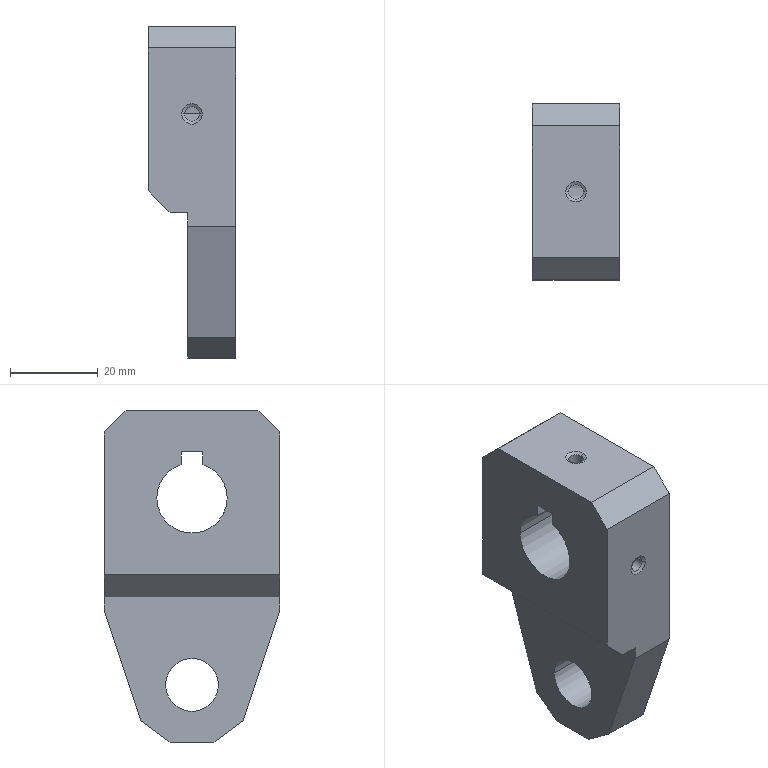Part | NX | 1 solid | 31 faces | box 20 x 40 x 75.5 mm | volume 38243 mm3 | plane 18 | cylinder 9 | cone 4 | commonest cylinder face diameters 3.3 x4 16 x3 12 x2
STEP:
#1=CARTESIAN_POINT('',(1874.,-5.,-55.5));
#2=VERTEX_POINT('',#1);
#3=CARTESIAN_POINT('',(1885.,-5.,-55.5));
#4=VERTEX_POINT('',#3);
#5=CARTESIAN_POINT('',(1879.5,-5.,-55.5));
#6=DIRECTION('',(1.,0.,0.));
#7=VECTOR('',#6,1000.);
#8=LINE('',#5,#7);
#9=EDGE_CURVE('',#2,#4,#8,.T.);
#10=ORIENTED_EDGE('',*,*,#9,.F.);
#11=CARTESIAN_POINT('',(1874.,5.,-55.5));
#12=VERTEX_POINT('',#11);
#13=CARTESIAN_POINT('',(1874.,-0.7647,-55.5));
#14=DIRECTION('',(0.,1.,0.));
#15=VECTOR('',#14,1000.);
#16=LINE('',#13,#15);
#17=EDGE_CURVE('',#2,#12,#16,.T.);
#18=ORIENTED_EDGE('',*,*,#17,.T.);
#19=CARTESIAN_POINT('',(1885.,5.,-55.5));
#20=VERTEX_POINT('',#19);
#21=CARTESIAN_POINT('',(1879.5,5.,-55.5));
#22=DIRECTION('',(-1.,0.,0.));
#23=VECTOR('',#22,1000.);
#24=LINE('',#21,#23);
#25=EDGE_CURVE('',#20,#12,#24,.T.);
#26=ORIENTED_EDGE('',*,*,#25,.F.);
#27=CARTESIAN_POINT('',(1885.,-0.7647,-55.5));
#28=DIRECTION('',(0.,1.,0.));
#29=VECTOR('',#28,1000.);
#30=LINE('',#27,#29);
#31=EDGE_CURVE('',#4,#20,#30,.T.);
#32=ORIENTED_EDGE('',*,*,#31,.F.);
#33=EDGE_LOOP('',(#10,#18,#26,#32));
#34=FACE_BOUND('',#33,.T.);
#35=CARTESIAN_POINT('',(1885.,-20.,-55.5));
#36=DIRECTION('',(0.,0.,-1.));
#37=DIRECTION('',(0.,-1.,0.));
#38=AXIS2_PLACEMENT_3D('',#35,#36,#37);
#39=PLANE('',#38);
#40=ADVANCED_FACE('',(#34),#39,.T.);
#41=CARTESIAN_POINT('',(1865.,-20.,15.));
#42=VERTEX_POINT('',#41);
#43=CARTESIAN_POINT('',(1885.,-20.,15.));
#44=VERTEX_POINT('',#43);
#45=CARTESIAN_POINT('',(0.,-20.,15.));
#46=DIRECTION('',(1.,0.,0.));
#47=VECTOR('',#46,1000.);
#48=LINE('',#45,#47);
#49=EDGE_CURVE('',#42,#44,#48,.T.);
#50=ORIENTED_EDGE('',*,*,#49,.F.);
#51=CARTESIAN_POINT('',(1865.,-20.,-17.5));
#52=VERTEX_POINT('',#51);
#53=CARTESIAN_POINT('',(1865.,-20.,0.));
#54=DIRECTION('',(0.,0.,-1.));
#55=VECTOR('',#54,1000.);
#56=LINE('',#53,#55);
#57=EDGE_CURVE('',#42,#52,#56,.T.);
#58=ORIENTED_EDGE('',*,*,#57,.T.);
#59=CARTESIAN_POINT('',(1870.,-20.,-22.5));
#60=VERTEX_POINT('',#59);
#61=CARTESIAN_POINT('',(1847.5,-20.,0.));
#62=DIRECTION('',(0.7071,0.,-0.7071));
#63=VECTOR('',#62,1000.);
#64=LINE('',#61,#63);
#65=EDGE_CURVE('',#52,#60,#64,.T.);
#66=ORIENTED_EDGE('',*,*,#65,.T.);
#67=CARTESIAN_POINT('',(1874.,-20.,-22.5));
#68=VERTEX_POINT('',#67);
#69=CARTESIAN_POINT('',(0.,-20.,-22.5));
#70=DIRECTION('',(1.,0.,0.));
#71=VECTOR('',#70,1000.);
#72=LINE('',#69,#71);
#73=EDGE_CURVE('',#60,#68,#72,.T.);
#74=ORIENTED_EDGE('',*,*,#73,.T.);
#75=CARTESIAN_POINT('',(1874.,-20.,-25.5));
#76=VERTEX_POINT('',#75);
#77=CARTESIAN_POINT('',(1874.,-20.,0.));
#78=DIRECTION('',(0.,0.,-1.));
#79=VECTOR('',#78,1000.);
#80=LINE('',#77,#79);
#81=EDGE_CURVE('',#68,#76,#80,.T.);
#82=ORIENTED_EDGE('',*,*,#81,.T.);
#83=CARTESIAN_POINT('',(1885.,-20.,-25.5));
#84=VERTEX_POINT('',#83);
#85=CARTESIAN_POINT('',(0.,-20.,-25.5));
#86=DIRECTION('',(1.,0.,0.));
#87=VECTOR('',#86,1000.);
#88=LINE('',#85,#87);
#89=EDGE_CURVE('',#76,#84,#88,.T.);
#90=ORIENTED_EDGE('',*,*,#89,.T.);
#91=CARTESIAN_POINT('',(1885.,-20.,0.));
#92=DIRECTION('',(0.,0.,-1.));
#93=VECTOR('',#92,1000.);
#94=LINE('',#91,#93);
#95=EDGE_CURVE('',#44,#84,#94,.T.);
#96=ORIENTED_EDGE('',*,*,#95,.F.);
#97=EDGE_LOOP('',(#50,#58,#66,#74,#82,#90,#96));
#98=FACE_BOUND('',#97,.T.);
#99=CARTESIAN_POINT('',(1877.315,-20.,0.));
#100=VERTEX_POINT('',#99);
#101=CARTESIAN_POINT('',(1872.685,-20.,0.));
#102=VERTEX_POINT('',#101);
#103=CARTESIAN_POINT('',(1875.,-20.,0.));
#104=DIRECTION('',(0.,-1.,0.));
#105=DIRECTION('',(-1.,0.,0.));
#106=AXIS2_PLACEMENT_3D('',#103,#104,#105);
#107=CIRCLE('',#106,2.315);
#108=EDGE_CURVE('',#100,#102,#107,.T.);
#109=ORIENTED_EDGE('',*,*,#108,.F.);
#110=CARTESIAN_POINT('',(1875.,-20.,0.));
#111=DIRECTION('',(0.,-1.,0.));
#112=DIRECTION('',(-1.,0.,0.));
#113=AXIS2_PLACEMENT_3D('',#110,#111,#112);
#114=CIRCLE('',#113,2.315);
#115=EDGE_CURVE('',#102,#100,#114,.T.);
#116=ORIENTED_EDGE('',*,*,#115,.F.);
#117=EDGE_LOOP('',(#109,#116));
#118=FACE_BOUND('',#117,.T.);
#119=CARTESIAN_POINT('',(1885.,-20.,20.));
#120=DIRECTION('',(0.,-1.,0.));
#121=DIRECTION('',(0.,0.,-1.));
#122=AXIS2_PLACEMENT_3D('',#119,#120,#121);
#123=PLANE('',#122);
#124=ADVANCED_FACE('',(#98,#118),#123,.T.);
#125=CARTESIAN_POINT('',(1865.,15.,20.));
#126=VERTEX_POINT('',#125);
#127=CARTESIAN_POINT('',(1885.,15.,20.));
#128=VERTEX_POINT('',#127);
#129=CARTESIAN_POINT('',(0.,15.,20.));
#130=DIRECTION('',(1.,0.,0.));
#131=VECTOR('',#130,1000.);
#132=LINE('',#129,#131);
#133=EDGE_CURVE('',#126,#128,#132,.T.);
#134=ORIENTED_EDGE('',*,*,#133,.F.);
#135=CARTESIAN_POINT('',(1865.,-15.,20.));
#136=VERTEX_POINT('',#135);
#137=CARTESIAN_POINT('',(1865.,0.,20.));
#138=DIRECTION('',(0.,-1.,0.));
#139=VECTOR('',#138,1000.);
#140=LINE('',#137,#139);
#141=EDGE_CURVE('',#126,#136,#140,.T.);
#142=ORIENTED_EDGE('',*,*,#141,.T.);
#143=CARTESIAN_POINT('',(1885.,-15.,20.));
#144=VERTEX_POINT('',#143);
#145=CARTESIAN_POINT('',(0.,-15.,20.));
#146=DIRECTION('',(-1.,0.,0.));
#147=VECTOR('',#146,1000.);
#148=LINE('',#145,#147);
#149=EDGE_CURVE('',#144,#136,#148,.T.);
#150=ORIENTED_EDGE('',*,*,#149,.F.);
#151=CARTESIAN_POINT('',(1885.,0.,20.));
#152=DIRECTION('',(0.,-1.,0.));
#153=VECTOR('',#152,1000.);
#154=LINE('',#151,#153);
#155=EDGE_CURVE('',#128,#144,#154,.T.);
#156=ORIENTED_EDGE('',*,*,#155,.F.);
#157=EDGE_LOOP('',(#134,#142,#150,#156));
#158=FACE_BOUND('',#157,.T.);
#159=CARTESIAN_POINT('',(1872.685,0.,20.));
#160=VERTEX_POINT('',#159);
#161=CARTESIAN_POINT('',(1877.315,0.,20.));
#162=VERTEX_POINT('',#161);
#163=CARTESIAN_POINT('',(1875.,0.,20.));
#164=DIRECTION('',(0.,0.,1.));
#165=DIRECTION('',(1.,0.,0.));
#166=AXIS2_PLACEMENT_3D('',#163,#164,#165);
#167=CIRCLE('',#166,2.315);
#168=EDGE_CURVE('',#160,#162,#167,.T.);
#169=ORIENTED_EDGE('',*,*,#168,.F.);
#170=CARTESIAN_POINT('',(1875.,0.,20.));
#171=DIRECTION('',(0.,0.,1.));
#172=DIRECTION('',(1.,0.,0.));
#173=AXIS2_PLACEMENT_3D('',#170,#171,#172);
#174=CIRCLE('',#173,2.315);
#175=EDGE_CURVE('',#162,#160,#174,.T.);
#176=ORIENTED_EDGE('',*,*,#175,.F.);
#177=EDGE_LOOP('',(#169,#176));
#178=FACE_BOUND('',#177,.T.);
#179=CARTESIAN_POINT('',(1885.,20.,20.));
#180=DIRECTION('',(0.,0.,1.));
#181=DIRECTION('',(1.,0.,0.));
#182=AXIS2_PLACEMENT_3D('',#179,#180,#181);
#183=PLANE('',#182);
#184=ADVANCED_FACE('',(#158,#178),#183,.T.);
#185=CARTESIAN_POINT('',(1870.,20.,-22.5));
#186=VERTEX_POINT('',#185);
#187=CARTESIAN_POINT('',(1874.,20.,-22.5));
#188=VERTEX_POINT('',#187);
#189=CARTESIAN_POINT('',(1885.,20.,-22.5));
#190=DIRECTION('',(1.,0.,0.));
#191=VECTOR('',#190,1000.);
#192=LINE('',#189,#191);
#193=EDGE_CURVE('',#186,#188,#192,.T.);
#194=ORIENTED_EDGE('',*,*,#193,.F.);
#195=CARTESIAN_POINT('',(1865.,20.,-17.5));
#196=VERTEX_POINT('',#195);
#197=CARTESIAN_POINT('',(1885.,20.,-37.5));
#198=DIRECTION('',(-0.7071,0.,0.7071));
#199=VECTOR('',#198,1000.);
#200=LINE('',#197,#199);
#201=EDGE_CURVE('',#186,#196,#200,.T.);
#202=ORIENTED_EDGE('',*,*,#201,.T.);
#203=CARTESIAN_POINT('',(1865.,20.,15.));
#204=VERTEX_POINT('',#203);
#205=CARTESIAN_POINT('',(1865.,20.,0.8535));
#206=DIRECTION('',(0.,0.,1.));
#207=VECTOR('',#206,1000.);
#208=LINE('',#205,#207);
#209=EDGE_CURVE('',#196,#204,#208,.T.);
#210=ORIENTED_EDGE('',*,*,#209,.T.);
#211=CARTESIAN_POINT('',(1885.,20.,15.));
#212=VERTEX_POINT('',#211);
#213=CARTESIAN_POINT('',(1875.,20.,15.));
#214=DIRECTION('',(-1.,0.,0.));
#215=VECTOR('',#214,1000.);
#216=LINE('',#213,#215);
#217=EDGE_CURVE('',#212,#204,#216,.T.);
#218=ORIENTED_EDGE('',*,*,#217,.F.);
#219=CARTESIAN_POINT('',(1885.,20.,-25.5));
#220=VERTEX_POINT('',#219);
#221=CARTESIAN_POINT('',(1885.,20.,0.8535));
#222=DIRECTION('',(0.,0.,1.));
#223=VECTOR('',#222,1000.);
#224=LINE('',#221,#223);
#225=EDGE_CURVE('',#220,#212,#224,.T.);
#226=ORIENTED_EDGE('',*,*,#225,.F.);
#227=CARTESIAN_POINT('',(1874.,20.,-25.5));
#228=VERTEX_POINT('',#227);
#229=CARTESIAN_POINT('',(1879.5,20.,-25.5));
#230=DIRECTION('',(-1.,0.,0.));
#231=VECTOR('',#230,1000.);
#232=LINE('',#229,#231);
#233=EDGE_CURVE('',#220,#228,#232,.T.);
#234=ORIENTED_EDGE('',*,*,#233,.T.);
#235=CARTESIAN_POINT('',(1874.,20.,0.8535));
#236=DIRECTION('',(0.,0.,1.));
#237=VECTOR('',#236,1000.);
#238=LINE('',#235,#237);
#239=EDGE_CURVE('',#228,#188,#238,.T.);
#240=ORIENTED_EDGE('',*,*,#239,.T.);
#241=EDGE_LOOP('',(#194,#202,#210,#218,#226,#234,#240));
#242=FACE_BOUND('',#241,.T.);
#243=CARTESIAN_POINT('',(1885.,20.,-62.5));
#244=DIRECTION('',(0.,1.,0.));
#245=DIRECTION('',(1.,0.,0.));
#246=AXIS2_PLACEMENT_3D('',#243,#244,#245);
#247=PLANE('',#246);
#248=ADVANCED_FACE('',(#242),#247,.T.);
#249=CARTESIAN_POINT('',(1870.,0.,-22.5));
#250=DIRECTION('',(0.,-1.,0.));
#251=VECTOR('',#250,1000.);
#252=LINE('',#249,#251);
#253=EDGE_CURVE('',#186,#60,#252,.T.);
#254=ORIENTED_EDGE('',*,*,#253,.F.);
#255=ORIENTED_EDGE('',*,*,#193,.T.);
#256=CARTESIAN_POINT('',(1874.,24.,-22.5));
#257=DIRECTION('',(0.,-1.,0.));
#258=VECTOR('',#257,1000.);
#259=LINE('',#256,#258);
#260=EDGE_CURVE('',#188,#68,#259,.T.);
#261=ORIENTED_EDGE('',*,*,#260,.T.);
#262=ORIENTED_EDGE('',*,*,#73,.F.);
#263=EDGE_LOOP('',(#254,#255,#261,#262));
#264=FACE_BOUND('',#263,.T.);
#265=CARTESIAN_POINT('',(1865.,24.,-22.5));
#266=DIRECTION('',(0.,0.,1.));
#267=DIRECTION('',(1.,0.,0.));
#268=AXIS2_PLACEMENT_3D('',#265,#266,#267);
#269=PLANE('',#268);
#270=ADVANCED_FACE('',(#264),#269,.F.);
#271=ORIENTED_EDGE('',*,*,#133,.T.);
#272=CARTESIAN_POINT('',(1885.,34.147,0.8535));
#273=DIRECTION('',(0.,0.7071,-0.7071));
#274=VECTOR('',#273,1000.);
#275=LINE('',#272,#274);
#276=EDGE_CURVE('',#128,#212,#275,.T.);
#277=ORIENTED_EDGE('',*,*,#276,.T.);
#278=ORIENTED_EDGE('',*,*,#217,.T.);
#279=CARTESIAN_POINT('',(1865.,34.147,0.8535));
#280=DIRECTION('',(0.,0.7071,-0.7071));
#281=VECTOR('',#280,1000.);
#282=LINE('',#279,#281);
#283=EDGE_CURVE('',#126,#204,#282,.T.);
#284=ORIENTED_EDGE('',*,*,#283,.F.);
#285=EDGE_LOOP('',(#271,#277,#278,#284));
#286=FACE_BOUND('',#285,.T.);
#287=CARTESIAN_POINT('',(1875.,17.5,17.5));
#288=DIRECTION('',(0.,0.7071,0.7071));
#289=DIRECTION('',(1.,0.,0.));
#290=AXIS2_PLACEMENT_3D('',#287,#288,#289);
#291=PLANE('',#290);
#292=ADVANCED_FACE('',(#286),#291,.T.);
#293=ORIENTED_EDGE('',*,*,#253,.T.);
#294=ORIENTED_EDGE('',*,*,#65,.F.);
#295=CARTESIAN_POINT('',(1865.,0.,-17.5));
#296=DIRECTION('',(0.,-1.,0.));
#297=VECTOR('',#296,1000.);
#298=LINE('',#295,#297);
#299=EDGE_CURVE('',#196,#52,#298,.T.);
#300=ORIENTED_EDGE('',*,*,#299,.F.);
#301=ORIENTED_EDGE('',*,*,#201,.F.);
#302=EDGE_LOOP('',(#293,#294,#300,#301));
#303=FACE_BOUND('',#302,.T.);
#304=CARTESIAN_POINT('',(1867.5,0.,-20.));
#305=DIRECTION('',(0.7071,0.,0.7071));
#306=DIRECTION('',(0.,-1.,0.));
#307=AXIS2_PLACEMENT_3D('',#304,#305,#306);
#308=PLANE('',#307);
#309=ADVANCED_FACE('',(#303),#308,.F.);
#310=CARTESIAN_POINT('',(1865.,2.5,7.599));
#311=VERTEX_POINT('',#310);
#312=CARTESIAN_POINT('',(1885.,2.5,7.599));
#313=VERTEX_POINT('',#312);
#314=CARTESIAN_POINT('',(1885.,2.5,7.599));
#315=DIRECTION('',(1.,0.,0.));
#316=VECTOR('',#315,1000.);
#317=LINE('',#314,#316);
#318=EDGE_CURVE('',#311,#313,#317,.T.);
#319=ORIENTED_EDGE('',*,*,#318,.T.);
#320=CARTESIAN_POINT('',(1885.,2.5,10.5));
#321=VERTEX_POINT('',#320);
#322=CARTESIAN_POINT('',(1885.,2.5,0.8535));
#323=DIRECTION('',(0.,0.,1.));
#324=VECTOR('',#323,1000.);
#325=LINE('',#322,#324);
#326=EDGE_CURVE('',#313,#321,#325,.T.);
#327=ORIENTED_EDGE('',*,*,#326,.T.);
#328=CARTESIAN_POINT('',(1865.,2.5,10.5));
#329=VERTEX_POINT('',#328);
#330=CARTESIAN_POINT('',(0.,2.5,10.5));
#331=DIRECTION('',(1.,0.,0.));
#332=VECTOR('',#331,1000.);
#333=LINE('',#330,#332);
#334=EDGE_CURVE('',#329,#321,#333,.T.);
#335=ORIENTED_EDGE('',*,*,#334,.F.);
#336=CARTESIAN_POINT('',(1865.,2.5,0.8535));
#337=DIRECTION('',(0.,0.,1.));
#338=VECTOR('',#337,1000.);
#339=LINE('',#336,#338);
#340=EDGE_CURVE('',#311,#329,#339,.T.);
#341=ORIENTED_EDGE('',*,*,#340,.F.);
#342=EDGE_LOOP('',(#319,#327,#335,#341));
#343=FACE_BOUND('',#342,.T.);
#344=CARTESIAN_POINT('',(1863.,2.5,10.5));
#345=DIRECTION('',(0.,1.,0.));
#346=DIRECTION('',(1.,0.,0.));
#347=AXIS2_PLACEMENT_3D('',#344,#345,#346);
#348=PLANE('',#347);
#349=ADVANCED_FACE('',(#343),#348,.F.);
#350=CARTESIAN_POINT('',(1885.,6.,-42.5));
#351=VERTEX_POINT('',#350);
#352=CARTESIAN_POINT('',(1885.,-6.,-42.5));
#353=VERTEX_POINT('',#352);
#354=CARTESIAN_POINT('',(1885.,0.,-42.5));
#355=DIRECTION('',(1.,0.,0.));
#356=DIRECTION('',(0.,1.,0.));
#357=AXIS2_PLACEMENT_3D('',#354,#355,#356);
#358=CIRCLE('',#357,6.);
#359=EDGE_CURVE('',#351,#353,#358,.T.);
#360=ORIENTED_EDGE('',*,*,#359,.T.);
#361=CARTESIAN_POINT('',(1874.,-6.,-42.5));
#362=VERTEX_POINT('',#361);
#363=CARTESIAN_POINT('',(1863.,-6.,-42.5));
#364=DIRECTION('',(1.,0.,0.));
#365=VECTOR('',#364,1000.);
#366=LINE('',#363,#365);
#367=EDGE_CURVE('',#353,#362,#366,.F.);
#368=ORIENTED_EDGE('',*,*,#367,.T.);
#369=CARTESIAN_POINT('',(1874.,6.,-42.5));
#370=VERTEX_POINT('',#369);
#371=CARTESIAN_POINT('',(1874.,0.,-42.5));
#372=DIRECTION('',(1.,0.,0.));
#373=DIRECTION('',(0.,1.,0.));
#374=AXIS2_PLACEMENT_3D('',#371,#372,#373);
#375=CIRCLE('',#374,6.);
#376=EDGE_CURVE('',#370,#362,#375,.T.);
#377=ORIENTED_EDGE('',*,*,#376,.F.);
#378=CARTESIAN_POINT('',(1863.,6.,-42.5));
#379=DIRECTION('',(1.,0.,0.));
#380=VECTOR('',#379,1000.);
#381=LINE('',#378,#380);
#382=EDGE_CURVE('',#351,#370,#381,.F.);
#383=ORIENTED_EDGE('',*,*,#382,.F.);
#384=EDGE_LOOP('',(#360,#368,#377,#383));
#385=FACE_BOUND('',#384,.T.);
#386=CARTESIAN_POINT('',(1863.,0.,-42.5));
#387=DIRECTION('',(1.,0.,0.));
#388=DIRECTION('',(0.,1.,0.));
#389=AXIS2_PLACEMENT_3D('',#386,#387,#388);
#390=CYLINDRICAL_SURFACE('',#389,6.);
#391=ADVANCED_FACE('',(#385),#390,.F.);
#392=CARTESIAN_POINT('',(1865.,-8.,0.));
#393=VERTEX_POINT('',#392);
#394=CARTESIAN_POINT('',(1873.35,-8.,0.));
#395=VERTEX_POINT('',#394);
#396=CARTESIAN_POINT('',(1885.,-8.,0.));
#397=DIRECTION('',(1.,0.,0.));
#398=VECTOR('',#397,1000.);
#399=LINE('',#396,#398);
#400=EDGE_CURVE('',#393,#395,#399,.T.);
#401=ORIENTED_EDGE('',*,*,#400,.F.);
#402=CARTESIAN_POINT('',(1865.,-2.5,7.599));
#403=VERTEX_POINT('',#402);
#404=CARTESIAN_POINT('',(1865.,0.,0.));
#405=DIRECTION('',(1.,0.,0.));
#406=DIRECTION('',(0.,1.,0.));
#407=AXIS2_PLACEMENT_3D('',#404,#405,#406);
#408=CIRCLE('',#407,8.);
#409=EDGE_CURVE('',#403,#393,#408,.T.);
#410=ORIENTED_EDGE('',*,*,#409,.F.);
#411=CARTESIAN_POINT('',(1885.,-2.5,7.599));
#412=VERTEX_POINT('',#411);
#413=CARTESIAN_POINT('',(1885.,-2.5,7.599));
#414=DIRECTION('',(1.,0.,0.));
#415=VECTOR('',#414,1000.);
#416=LINE('',#413,#415);
#417=EDGE_CURVE('',#403,#412,#416,.T.);
#418=ORIENTED_EDGE('',*,*,#417,.T.);
#419=CARTESIAN_POINT('',(1885.,-8.,0.));
#420=VERTEX_POINT('',#419);
#421=CARTESIAN_POINT('',(1885.,0.,0.));
#422=DIRECTION('',(1.,0.,0.));
#423=DIRECTION('',(0.,1.,0.));
#424=AXIS2_PLACEMENT_3D('',#421,#422,#423);
#425=CIRCLE('',#424,8.);
#426=EDGE_CURVE('',#412,#420,#425,.T.);
#427=ORIENTED_EDGE('',*,*,#426,.T.);
#428=CARTESIAN_POINT('',(1876.65,-8.,0.));
#429=VERTEX_POINT('',#428);
#430=CARTESIAN_POINT('',(1885.,-8.,0.));
#431=DIRECTION('',(1.,0.,0.));
#432=VECTOR('',#431,1000.);
#433=LINE('',#430,#432);
#434=EDGE_CURVE('',#429,#420,#433,.T.);
#435=ORIENTED_EDGE('',*,*,#434,.F.);
#436=CARTESIAN_POINT('',(1875.,-7.828,1.65));
#437=VERTEX_POINT('',#436);
#438=CARTESIAN_POINT('',(1876.65,-8.,0.));
#439=CARTESIAN_POINT('',(1876.65,-8.,0.05388));
#440=CARTESIAN_POINT('',(1876.647,-7.999,0.1078));
#441=CARTESIAN_POINT('',(1876.642,-7.998,0.1614));
#442=CARTESIAN_POINT('',(1876.639,-7.998,0.1882));
#443=CARTESIAN_POINT('',(1876.636,-7.997,0.2149));
#444=CARTESIAN_POINT('',(1876.632,-7.996,0.2416));
#445=CARTESIAN_POINT('',(1876.628,-7.996,0.2682));
#446=CARTESIAN_POINT('',(1876.624,-7.995,0.2948));
#447=CARTESIAN_POINT('',(1876.618,-7.994,0.3212));
#448=CARTESIAN_POINT('',(1876.613,-7.992,0.3476));
#449=CARTESIAN_POINT('',(1876.607,-7.991,0.3739));
#450=CARTESIAN_POINT('',(1876.601,-7.99,0.4));
#451=CARTESIAN_POINT('',(1876.594,-7.989,0.4262));
#452=CARTESIAN_POINT('',(1876.587,-7.987,0.4522));
#453=CARTESIAN_POINT('',(1876.579,-7.986,0.4779));
#454=CARTESIAN_POINT('',(1876.571,-7.984,0.5037));
#455=CARTESIAN_POINT('',(1876.563,-7.983,0.5292));
#456=CARTESIAN_POINT('',(1876.554,-7.981,0.5546));
#457=CARTESIAN_POINT('',(1876.545,-7.979,0.5799));
#458=CARTESIAN_POINT('',(1876.535,-7.977,0.6051));
#459=CARTESIAN_POINT('',(1876.525,-7.975,0.63));
#460=CARTESIAN_POINT('',(1876.515,-7.973,0.655));
#461=CARTESIAN_POINT('',(1876.504,-7.971,0.6797));
#462=CARTESIAN_POINT('',(1876.492,-7.969,0.7042));
#463=CARTESIAN_POINT('',(1876.481,-7.967,0.7287));
#464=CARTESIAN_POINT('',(1876.468,-7.965,0.7529));
#465=CARTESIAN_POINT('',(1876.456,-7.962,0.7768));
#466=CARTESIAN_POINT('',(1876.443,-7.96,0.8007));
#467=CARTESIAN_POINT('',(1876.43,-7.957,0.8242));
#468=CARTESIAN_POINT('',(1876.416,-7.955,0.8475));
#469=CARTESIAN_POINT('',(1876.402,-7.953,0.8707));
#470=CARTESIAN_POINT('',(1876.387,-7.95,0.8936));
#471=CARTESIAN_POINT('',(1876.372,-7.947,0.9161));
#472=CARTESIAN_POINT('',(1876.357,-7.945,0.9386));
#473=CARTESIAN_POINT('',(1876.342,-7.942,0.9607));
#474=CARTESIAN_POINT('',(1876.326,-7.939,0.9824));
#475=CARTESIAN_POINT('',(1876.31,-7.937,1.004));
#476=CARTESIAN_POINT('',(1876.293,-7.934,1.025));
#477=CARTESIAN_POINT('',(1876.276,-7.931,1.046));
#478=CARTESIAN_POINT('',(1876.259,-7.929,1.067));
#479=CARTESIAN_POINT('',(1876.242,-7.926,1.087));
#480=CARTESIAN_POINT('',(1876.224,-7.923,1.107));
#481=CARTESIAN_POINT('',(1876.206,-7.92,1.127));
#482=CARTESIAN_POINT('',(1876.187,-7.917,1.146));
#483=CARTESIAN_POINT('',(1876.168,-7.915,1.166));
#484=CARTESIAN_POINT('',(1876.149,-7.912,1.185));
#485=CARTESIAN_POINT('',(1876.129,-7.909,1.203));
#486=CARTESIAN_POINT('',(1876.109,-7.906,1.221));
#487=CARTESIAN_POINT('',(1876.089,-7.903,1.24));
#488=CARTESIAN_POINT('',(1876.069,-7.901,1.257));
#489=CARTESIAN_POINT('',(1876.048,-7.898,1.274));
#490=CARTESIAN_POINT('',(1876.027,-7.895,1.292));
#491=CARTESIAN_POINT('',(1876.006,-7.892,1.308));
#492=CARTESIAN_POINT('',(1875.984,-7.89,1.324));
#493=CARTESIAN_POINT('',(1875.962,-7.887,1.341));
#494=CARTESIAN_POINT('',(1875.94,-7.884,1.356));
#495=CARTESIAN_POINT('',(1875.918,-7.882,1.371));
#496=CARTESIAN_POINT('',(1875.895,-7.879,1.386));
#497=CARTESIAN_POINT('',(1875.872,-7.876,1.401));
#498=CARTESIAN_POINT('',(1875.849,-7.874,1.415));
#499=CARTESIAN_POINT('',(1875.826,-7.871,1.429));
#500=CARTESIAN_POINT('',(1875.803,-7.869,1.442));
#501=CARTESIAN_POINT('',(1875.779,-7.867,1.455));
#502=CARTESIAN_POINT('',(1875.755,-7.864,1.467));
#503=CARTESIAN_POINT('',(1875.731,-7.862,1.479));
#504=CARTESIAN_POINT('',(1875.707,-7.86,1.491));
#505=CARTESIAN_POINT('',(1875.683,-7.858,1.502));
#506=CARTESIAN_POINT('',(1875.658,-7.856,1.513));
#507=CARTESIAN_POINT('',(1875.633,-7.854,1.524));
#508=CARTESIAN_POINT('',(1875.608,-7.852,1.534));
#509=CARTESIAN_POINT('',(1875.583,-7.85,1.544));
#510=CARTESIAN_POINT('',(1875.557,-7.848,1.553));
#511=CARTESIAN_POINT('',(1875.532,-7.846,1.562));
#512=CARTESIAN_POINT('',(1875.506,-7.844,1.571));
#513=CARTESIAN_POINT('',(1875.48,-7.843,1.579));
#514=CARTESIAN_POINT('',(1875.454,-7.841,1.586));
#515=CARTESIAN_POINT('',(1875.428,-7.84,1.594));
#516=CARTESIAN_POINT('',(1875.402,-7.838,1.6));
#517=CARTESIAN_POINT('',(1875.375,-7.837,1.607));
#518=CARTESIAN_POINT('',(1875.349,-7.836,1.613));
#519=CARTESIAN_POINT('',(1875.322,-7.835,1.618));
#520=CARTESIAN_POINT('',(1875.296,-7.834,1.624));
#521=CARTESIAN_POINT('',(1875.269,-7.833,1.628));
#522=CARTESIAN_POINT('',(1875.242,-7.832,1.632));
#523=CARTESIAN_POINT('',(1875.215,-7.831,1.636));
#524=CARTESIAN_POINT('',(1875.188,-7.83,1.639));
#525=CARTESIAN_POINT('',(1875.161,-7.83,1.642));
#526=CARTESIAN_POINT('',(1875.135,-7.829,1.645));
#527=CARTESIAN_POINT('',(1875.108,-7.829,1.647));
#528=CARTESIAN_POINT('',(1875.081,-7.828,1.648));
#529=CARTESIAN_POINT('',(1875.054,-7.828,1.649));
#530=CARTESIAN_POINT('',(1875.027,-7.828,1.65));
#531=CARTESIAN_POINT('',(1875.,-7.828,1.65));
#532=B_SPLINE_CURVE_WITH_KNOTS('',3,(#438,#439,#440,#441,#442,#443,#444,#445,#446,#447,#448,#449,#450,#451,#452,#453,#454,#455,#456,#457,#458,#459,#460,#461,#462,#463,#464,#465,#466,#467,#468,#469,#470,#471,#472,#473,#474,#475,#476,#477,#478,#479,#480,#481,#482,#483,#484,#485,#486,#487,#488,#489,#490,#491,#492,#493,#494,#495,#496,#497,#498,#499,#500,#501,#502,#503,#504,#505,#506,#507,#508,#509,#510,#511,#512,#513,#514,#515,#516,#517,#518,#519,#520,#521,#522,#523,#524,#525,#526,#527,#528,#529,#530,#531),.UNSPECIFIED.,.F.,.F.,(4,3,3,3,3,3,3,3,3,3,3,3,3,3,3,3,3,3,3,3,3,3,3,3,3,3,3,3,3,3,3,4),(0.,0.1617,0.2425,0.3233,0.4042,0.4852,0.566,0.6471,0.7284,0.8099,0.8915,0.973,1.054,1.136,1.217,1.298,1.379,1.461,1.542,1.624,1.705,1.786,1.867,1.948,2.03,2.111,2.193,2.274,2.356,2.437,2.518,2.599),.UNSPECIFIED.);
#533=EDGE_CURVE('',#429,#437,#532,.T.);
#534=ORIENTED_EDGE('',*,*,#533,.T.);
#535=CARTESIAN_POINT('',(1875.,-7.828,1.65));
#536=CARTESIAN_POINT('',(1874.973,-7.828,1.65));
#537=CARTESIAN_POINT('',(1874.946,-7.828,1.649));
#538=CARTESIAN_POINT('',(1874.919,-7.828,1.648));
#539=CARTESIAN_POINT('',(1874.892,-7.829,1.647));
#540=CARTESIAN_POINT('',(1874.865,-7.829,1.645));
#541=CARTESIAN_POINT('',(1874.838,-7.83,1.642));
#542=CARTESIAN_POINT('',(1874.811,-7.83,1.639));
#543=CARTESIAN_POINT('',(1874.784,-7.831,1.636));
#544=CARTESIAN_POINT('',(1874.757,-7.832,1.632));
#545=CARTESIAN_POINT('',(1874.73,-7.833,1.628));
#546=CARTESIAN_POINT('',(1874.704,-7.834,1.623));
#547=CARTESIAN_POINT('',(1874.677,-7.835,1.618));
#548=CARTESIAN_POINT('',(1874.65,-7.836,1.613));
#549=CARTESIAN_POINT('',(1874.624,-7.837,1.607));
#550=CARTESIAN_POINT('',(1874.597,-7.838,1.6));
#551=CARTESIAN_POINT('',(1874.571,-7.84,1.594));
#552=CARTESIAN_POINT('',(1874.545,-7.841,1.586));
#553=CARTESIAN_POINT('',(1874.519,-7.843,1.578));
#554=CARTESIAN_POINT('',(1874.493,-7.844,1.57));
#555=CARTESIAN_POINT('',(1874.467,-7.846,1.562));
#556=CARTESIAN_POINT('',(1874.442,-7.848,1.553));
#557=CARTESIAN_POINT('',(1874.417,-7.85,1.544));
#558=CARTESIAN_POINT('',(1874.392,-7.852,1.534));
#559=CARTESIAN_POINT('',(1874.367,-7.854,1.524));
#560=CARTESIAN_POINT('',(1874.342,-7.856,1.513));
#561=CARTESIAN_POINT('',(1874.317,-7.858,1.502));
#562=CARTESIAN_POINT('',(1874.293,-7.86,1.491));
#563=CARTESIAN_POINT('',(1874.269,-7.862,1.479));
#564=CARTESIAN_POINT('',(1874.245,-7.864,1.467));
#565=CARTESIAN_POINT('',(1874.221,-7.867,1.454));
#566=CARTESIAN_POINT('',(1874.197,-7.869,1.442));
#567=CARTESIAN_POINT('',(1874.173,-7.871,1.428));
#568=CARTESIAN_POINT('',(1874.15,-7.874,1.414));
#569=CARTESIAN_POINT('',(1874.127,-7.877,1.4));
#570=CARTESIAN_POINT('',(1874.104,-7.879,1.386));
#571=CARTESIAN_POINT('',(1874.082,-7.882,1.371));
#572=CARTESIAN_POINT('',(1874.059,-7.884,1.356));
#573=CARTESIAN_POINT('',(1874.037,-7.887,1.34));
#574=CARTESIAN_POINT('',(1874.015,-7.89,1.324));
#575=CARTESIAN_POINT('',(1873.994,-7.892,1.308));
#576=CARTESIAN_POINT('',(1873.972,-7.895,1.291));
#577=CARTESIAN_POINT('',(1873.951,-7.898,1.274));
#578=CARTESIAN_POINT('',(1873.931,-7.901,1.257));
#579=CARTESIAN_POINT('',(1873.91,-7.903,1.239));
#580=CARTESIAN_POINT('',(1873.89,-7.906,1.221));
#581=CARTESIAN_POINT('',(1873.87,-7.909,1.203));
#582=CARTESIAN_POINT('',(1873.851,-7.912,1.184));
#583=CARTESIAN_POINT('',(1873.832,-7.915,1.165));
#584=CARTESIAN_POINT('',(1873.813,-7.917,1.146));
#585=CARTESIAN_POINT('',(1873.795,-7.92,1.127));
#586=CARTESIAN_POINT('',(1873.777,-7.923,1.107));
#587=CARTESIAN_POINT('',(1873.758,-7.926,1.087));
#588=CARTESIAN_POINT('',(1873.741,-7.929,1.067));
#589=CARTESIAN_POINT('',(1873.724,-7.931,1.046));
#590=CARTESIAN_POINT('',(1873.707,-7.934,1.025));
#591=CARTESIAN_POINT('',(1873.69,-7.937,1.004));
#592=CARTESIAN_POINT('',(1873.674,-7.94,0.9819));
#593=CARTESIAN_POINT('',(1873.658,-7.942,0.9601));
#594=CARTESIAN_POINT('',(1873.642,-7.945,0.938));
#595=CARTESIAN_POINT('',(1873.627,-7.947,0.9155));
#596=CARTESIAN_POINT('',(1873.612,-7.95,0.8929));
#597=CARTESIAN_POINT('',(1873.598,-7.953,0.87));
#598=CARTESIAN_POINT('',(1873.584,-7.955,0.8468));
#599=CARTESIAN_POINT('',(1873.57,-7.958,0.8236));
#600=CARTESIAN_POINT('',(1873.557,-7.96,0.8));
#601=CARTESIAN_POINT('',(1873.544,-7.962,0.7762));
#602=CARTESIAN_POINT('',(1873.531,-7.965,0.7523));
#603=CARTESIAN_POINT('',(1873.519,-7.967,0.7282));
#604=CARTESIAN_POINT('',(1873.508,-7.969,0.7038));
#605=CARTESIAN_POINT('',(1873.496,-7.971,0.6794));
#606=CARTESIAN_POINT('',(1873.485,-7.973,0.6547));
#607=CARTESIAN_POINT('',(1873.475,-7.975,0.6299));
#608=CARTESIAN_POINT('',(1873.465,-7.977,0.6051));
#609=CARTESIAN_POINT('',(1873.455,-7.979,0.58));
#610=CARTESIAN_POINT('',(1873.446,-7.981,0.5546));
#611=CARTESIAN_POINT('',(1873.437,-7.983,0.5293));
#612=CARTESIAN_POINT('',(1873.429,-7.984,0.5037));
#613=CARTESIAN_POINT('',(1873.421,-7.986,0.4779));
#614=CARTESIAN_POINT('',(1873.413,-7.987,0.4521));
#615=CARTESIAN_POINT('',(1873.406,-7.989,0.4261));
#616=CARTESIAN_POINT('',(1873.399,-7.99,0.3999));
#617=CARTESIAN_POINT('',(1873.393,-7.991,0.3738));
#618=CARTESIAN_POINT('',(1873.387,-7.992,0.3475));
#619=CARTESIAN_POINT('',(1873.382,-7.994,0.3211));
#620=CARTESIAN_POINT('',(1873.376,-7.995,0.2947));
#621=CARTESIAN_POINT('',(1873.372,-7.996,0.2682));
#622=CARTESIAN_POINT('',(1873.368,-7.996,0.2415));
#623=CARTESIAN_POINT('',(1873.364,-7.997,0.2149));
#624=CARTESIAN_POINT('',(1873.361,-7.998,0.1882));
#625=CARTESIAN_POINT('',(1873.358,-7.998,0.1614));
#626=CARTESIAN_POINT('',(1873.353,-7.999,0.1077));
#627=CARTESIAN_POINT('',(1873.35,-8.,0.05387));
#628=CARTESIAN_POINT('',(1873.35,-8.,0.));
#629=B_SPLINE_CURVE_WITH_KNOTS('',3,(#535,#536,#537,#538,#539,#540,#541,#542,#543,#544,#545,#546,#547,#548,#549,#550,#551,#552,#553,#554,#555,#556,#557,#558,#559,#560,#561,#562,#563,#564,#565,#566,#567,#568,#569,#570,#571,#572,#573,#574,#575,#576,#577,#578,#579,#580,#581,#582,#583,#584,#585,#586,#587,#588,#589,#590,#591,#592,#593,#594,#595,#596,#597,#598,#599,#600,#601,#602,#603,#604,#605,#606,#607,#608,#609,#610,#611,#612,#613,#614,#615,#616,#617,#618,#619,#620,#621,#622,#623,#624,#625,#626,#627,#628),.UNSPECIFIED.,.F.,.F.,(4,3,3,3,3,3,3,3,3,3,3,3,3,3,3,3,3,3,3,3,3,3,3,3,3,3,3,3,3,3,3,4),(0.,0.08097,0.1622,0.2437,0.3253,0.4069,0.4884,0.5696,0.6506,0.7316,0.8129,0.8943,0.9759,1.058,1.139,1.22,1.301,1.382,1.464,1.545,1.627,1.708,1.79,1.871,1.952,2.033,2.114,2.195,2.276,2.356,2.437,2.599),.UNSPECIFIED.);
#630=EDGE_CURVE('',#437,#395,#629,.T.);
#631=ORIENTED_EDGE('',*,*,#630,.T.);
#632=EDGE_LOOP('',(#401,#410,#418,#427,#435,#534,#631));
#633=FACE_BOUND('',#632,.T.);
#634=CARTESIAN_POINT('',(1885.,0.,0.));
#635=DIRECTION('',(1.,0.,0.));
#636=DIRECTION('',(0.,1.,0.));
#637=AXIS2_PLACEMENT_3D('',#634,#635,#636);
#638=CYLINDRICAL_SURFACE('',#637,8.);
#639=ADVANCED_FACE('',(#633),#638,.F.);
#640=ORIENTED_EDGE('',*,*,#299,.T.);
#641=ORIENTED_EDGE('',*,*,#57,.F.);
#642=CARTESIAN_POINT('',(1865.,-34.147,0.8535));
#643=DIRECTION('',(0.,0.7071,0.7071));
#644=VECTOR('',#643,1000.);
#645=LINE('',#642,#644);
#646=EDGE_CURVE('',#42,#136,#645,.T.);
#647=ORIENTED_EDGE('',*,*,#646,.T.);
#648=ORIENTED_EDGE('',*,*,#141,.F.);
#649=ORIENTED_EDGE('',*,*,#283,.T.);
#650=ORIENTED_EDGE('',*,*,#209,.F.);
#651=EDGE_LOOP('',(#640,#641,#647,#648,#649,#650));
#652=FACE_BOUND('',#651,.T.);
#653=ORIENTED_EDGE('',*,*,#409,.T.);
#654=CARTESIAN_POINT('',(1865.,8.,0.));
#655=VERTEX_POINT('',#654);
#656=CARTESIAN_POINT('',(1865.,0.,0.));
#657=DIRECTION('',(1.,0.,0.));
#658=DIRECTION('',(0.,1.,0.));
#659=AXIS2_PLACEMENT_3D('',#656,#657,#658);
#660=CIRCLE('',#659,8.);
#661=EDGE_CURVE('',#393,#655,#660,.T.);
#662=ORIENTED_EDGE('',*,*,#661,.T.);
#663=CARTESIAN_POINT('',(1865.,0.,0.));
#664=DIRECTION('',(1.,0.,0.));
#665=DIRECTION('',(0.,1.,0.));
#666=AXIS2_PLACEMENT_3D('',#663,#664,#665);
#667=CIRCLE('',#666,8.);
#668=EDGE_CURVE('',#655,#311,#667,.T.);
#669=ORIENTED_EDGE('',*,*,#668,.T.);
#670=ORIENTED_EDGE('',*,*,#340,.T.);
#671=CARTESIAN_POINT('',(1865.,-2.5,10.5));
#672=VERTEX_POINT('',#671);
#673=CARTESIAN_POINT('',(1865.,0.,10.5));
#674=DIRECTION('',(0.,-1.,0.));
#675=VECTOR('',#674,1000.);
#676=LINE('',#673,#675);
#677=EDGE_CURVE('',#329,#672,#676,.T.);
#678=ORIENTED_EDGE('',*,*,#677,.T.);
#679=CARTESIAN_POINT('',(1865.,-2.5,0.8535));
#680=DIRECTION('',(0.,0.,-1.));
#681=VECTOR('',#680,1000.);
#682=LINE('',#679,#681);
#683=EDGE_CURVE('',#672,#403,#682,.T.);
#684=ORIENTED_EDGE('',*,*,#683,.T.);
#685=EDGE_LOOP('',(#653,#662,#669,#670,#678,#684));
#686=FACE_BOUND('',#685,.T.);
#687=CARTESIAN_POINT('',(1865.,-0.7647,0.8535));
#688=DIRECTION('',(1.,0.,0.));
#689=DIRECTION('',(0.,1.,0.));
#690=AXIS2_PLACEMENT_3D('',#687,#688,#689);
#691=PLANE('',#690);
#692=ADVANCED_FACE('',(#652,#686),#691,.F.);
#693=ORIENTED_EDGE('',*,*,#49,.T.);
#694=CARTESIAN_POINT('',(1885.,-34.147,0.8535));
#695=DIRECTION('',(0.,0.7071,0.7071));
#696=VECTOR('',#695,1000.);
#697=LINE('',#694,#696);
#698=EDGE_CURVE('',#44,#144,#697,.T.);
#699=ORIENTED_EDGE('',*,*,#698,.T.);
#700=ORIENTED_EDGE('',*,*,#149,.T.);
#701=ORIENTED_EDGE('',*,*,#646,.F.);
#702=EDGE_LOOP('',(#693,#699,#700,#701));
#703=FACE_BOUND('',#702,.T.);
#704=CARTESIAN_POINT('',(1875.,-17.5,17.5));
#705=DIRECTION('',(0.,-0.7071,0.7071));
#706=DIRECTION('',(-1.,0.,0.));
#707=AXIS2_PLACEMENT_3D('',#704,#705,#706);
#708=PLANE('',#707);
#709=ADVANCED_FACE('',(#703),#708,.T.);
#710=CARTESIAN_POINT('',(1885.,11.581,-50.757));
#711=VERTEX_POINT('',#710);
#712=CARTESIAN_POINT('',(1874.,11.581,-50.757));
#713=VERTEX_POINT('',#712);
#714=CARTESIAN_POINT('',(1879.5,11.581,-50.757));
#715=DIRECTION('',(-1.,0.,0.));
#716=VECTOR('',#715,1000.);
#717=LINE('',#714,#716);
#718=EDGE_CURVE('',#711,#713,#717,.T.);
#719=ORIENTED_EDGE('',*,*,#718,.T.);
#720=CARTESIAN_POINT('',(1874.,28.784,0.8535));
#721=DIRECTION('',(0.,0.3162,0.9487));
#722=VECTOR('',#721,1000.);
#723=LINE('',#720,#722);
#724=EDGE_CURVE('',#713,#228,#723,.T.);
#725=ORIENTED_EDGE('',*,*,#724,.T.);
#726=ORIENTED_EDGE('',*,*,#233,.F.);
#727=CARTESIAN_POINT('',(1885.,28.784,0.8535));
#728=DIRECTION('',(0.,0.3162,0.9487));
#729=VECTOR('',#728,1000.);
#730=LINE('',#727,#729);
#731=EDGE_CURVE('',#711,#220,#730,.T.);
#732=ORIENTED_EDGE('',*,*,#731,.F.);
#733=EDGE_LOOP('',(#719,#725,#726,#732));
#734=FACE_BOUND('',#733,.T.);
#735=CARTESIAN_POINT('',(1879.5,15.,-40.5));
#736=DIRECTION('',(0.,-0.9487,0.3162));
#737=DIRECTION('',(-1.,0.,0.));
#738=AXIS2_PLACEMENT_3D('',#735,#736,#737);
#739=PLANE('',#738);
#740=ADVANCED_FACE('',(#734),#739,.F.);
#741=CARTESIAN_POINT('',(1874.,-11.581,-50.757));
#742=VERTEX_POINT('',#741);
#743=CARTESIAN_POINT('',(1885.,-11.581,-50.757));
#744=VERTEX_POINT('',#743);
#745=CARTESIAN_POINT('',(1879.5,-11.581,-50.757));
#746=DIRECTION('',(1.,0.,0.));
#747=VECTOR('',#746,1000.);
#748=LINE('',#745,#747);
#749=EDGE_CURVE('',#742,#744,#748,.T.);
#750=ORIENTED_EDGE('',*,*,#749,.T.);
#751=CARTESIAN_POINT('',(1885.,-28.784,0.8535));
#752=DIRECTION('',(0.,0.3162,-0.9487));
#753=VECTOR('',#752,1000.);
#754=LINE('',#751,#753);
#755=EDGE_CURVE('',#84,#744,#754,.T.);
#756=ORIENTED_EDGE('',*,*,#755,.F.);
#757=ORIENTED_EDGE('',*,*,#89,.F.);
#758=CARTESIAN_POINT('',(1874.,-28.784,0.8535));
#759=DIRECTION('',(0.,0.3162,-0.9487));
#760=VECTOR('',#759,1000.);
#761=LINE('',#758,#760);
#762=EDGE_CURVE('',#76,#742,#761,.T.);
#763=ORIENTED_EDGE('',*,*,#762,.T.);
#764=EDGE_LOOP('',(#750,#756,#757,#763));
#765=FACE_BOUND('',#764,.T.);
#766=CARTESIAN_POINT('',(1879.5,-15.,-40.5));
#767=DIRECTION('',(0.,0.9487,0.3162));
#768=DIRECTION('',(1.,0.,0.));
#769=AXIS2_PLACEMENT_3D('',#766,#767,#768);
#770=PLANE('',#769);
#771=ADVANCED_FACE('',(#765),#770,.F.);
#772=ORIENTED_EDGE('',*,*,#25,.T.);
#773=CARTESIAN_POINT('',(1874.,-0.7647,-59.655));
#774=DIRECTION('',(0.,0.8112,0.5847));
#775=VECTOR('',#774,1000.);
#776=LINE('',#773,#775);
#777=EDGE_CURVE('',#12,#713,#776,.T.);
#778=ORIENTED_EDGE('',*,*,#777,.T.);
#779=ORIENTED_EDGE('',*,*,#718,.F.);
#780=CARTESIAN_POINT('',(1885.,-0.7647,-59.655));
#781=DIRECTION('',(0.,0.8112,0.5847));
#782=VECTOR('',#781,1000.);
#783=LINE('',#780,#782);
#784=EDGE_CURVE('',#20,#711,#783,.T.);
#785=ORIENTED_EDGE('',*,*,#784,.F.);
#786=EDGE_LOOP('',(#772,#778,#779,#785));
#787=FACE_BOUND('',#786,.T.);
#788=CARTESIAN_POINT('',(1879.5,8.291,-53.128));
#789=DIRECTION('',(0.,-0.5847,0.8112));
#790=DIRECTION('',(-1.,0.,0.));
#791=AXIS2_PLACEMENT_3D('',#788,#789,#790);
#792=PLANE('',#791);
#793=ADVANCED_FACE('',(#787),#792,.F.);
#794=ORIENTED_EDGE('',*,*,#9,.T.);
#795=CARTESIAN_POINT('',(1885.,-0.7647,-58.553));
#796=DIRECTION('',(0.,0.8112,-0.5847));
#797=VECTOR('',#796,1000.);
#798=LINE('',#795,#797);
#799=EDGE_CURVE('',#744,#4,#798,.T.);
#800=ORIENTED_EDGE('',*,*,#799,.F.);
#801=ORIENTED_EDGE('',*,*,#749,.F.);
#802=CARTESIAN_POINT('',(1874.,-0.7647,-58.553));
#803=DIRECTION('',(0.,0.8112,-0.5847));
#804=VECTOR('',#803,1000.);
#805=LINE('',#802,#804);
#806=EDGE_CURVE('',#742,#2,#805,.T.);
#807=ORIENTED_EDGE('',*,*,#806,.T.);
#808=EDGE_LOOP('',(#794,#800,#801,#807));
#809=FACE_BOUND('',#808,.T.);
#810=CARTESIAN_POINT('',(1879.5,-8.291,-53.128));
#811=DIRECTION('',(0.,0.5847,0.8112));
#812=DIRECTION('',(1.,0.,0.));
#813=AXIS2_PLACEMENT_3D('',#810,#811,#812);
#814=PLANE('',#813);
#815=ADVANCED_FACE('',(#809),#814,.F.);
#816=ORIENTED_EDGE('',*,*,#225,.T.);
#817=ORIENTED_EDGE('',*,*,#276,.F.);
#818=ORIENTED_EDGE('',*,*,#155,.T.);
#819=ORIENTED_EDGE('',*,*,#698,.F.);
#820=ORIENTED_EDGE('',*,*,#95,.T.);
#821=ORIENTED_EDGE('',*,*,#755,.T.);
#822=ORIENTED_EDGE('',*,*,#799,.T.);
#823=ORIENTED_EDGE('',*,*,#31,.T.);
#824=ORIENTED_EDGE('',*,*,#784,.T.);
#825=ORIENTED_EDGE('',*,*,#731,.T.);
#826=EDGE_LOOP('',(#816,#817,#818,#819,#820,#821,#822,#823,#824,#825));
#827=FACE_BOUND('',#826,.T.);
#828=ORIENTED_EDGE('',*,*,#359,.F.);
#829=CARTESIAN_POINT('',(1885.,0.,-42.5));
#830=DIRECTION('',(1.,0.,0.));
#831=DIRECTION('',(0.,1.,0.));
#832=AXIS2_PLACEMENT_3D('',#829,#830,#831);
#833=CIRCLE('',#832,6.);
#834=EDGE_CURVE('',#353,#351,#833,.T.);
#835=ORIENTED_EDGE('',*,*,#834,.F.);
#836=EDGE_LOOP('',(#828,#835));
#837=FACE_BOUND('',#836,.T.);
#838=ORIENTED_EDGE('',*,*,#426,.F.);
#839=CARTESIAN_POINT('',(1885.,-2.5,10.5));
#840=VERTEX_POINT('',#839);
#841=CARTESIAN_POINT('',(1885.,-2.5,0.8535));
#842=DIRECTION('',(0.,0.,-1.));
#843=VECTOR('',#842,1000.);
#844=LINE('',#841,#843);
#845=EDGE_CURVE('',#840,#412,#844,.T.);
#846=ORIENTED_EDGE('',*,*,#845,.F.);
#847=CARTESIAN_POINT('',(1885.,0.,10.5));
#848=DIRECTION('',(0.,-1.,0.));
#849=VECTOR('',#848,1000.);
#850=LINE('',#847,#849);
#851=EDGE_CURVE('',#321,#840,#850,.T.);
#852=ORIENTED_EDGE('',*,*,#851,.F.);
#853=ORIENTED_EDGE('',*,*,#326,.F.);
#854=CARTESIAN_POINT('',(1885.,8.,0.));
#855=VERTEX_POINT('',#854);
#856=CARTESIAN_POINT('',(1885.,0.,0.));
#857=DIRECTION('',(1.,0.,0.));
#858=DIRECTION('',(0.,1.,0.));
#859=AXIS2_PLACEMENT_3D('',#856,#857,#858);
#860=CIRCLE('',#859,8.);
#861=EDGE_CURVE('',#855,#313,#860,.T.);
#862=ORIENTED_EDGE('',*,*,#861,.F.);
#863=CARTESIAN_POINT('',(1885.,0.,0.));
#864=DIRECTION('',(1.,0.,0.));
#865=DIRECTION('',(0.,1.,0.));
#866=AXIS2_PLACEMENT_3D('',#863,#864,#865);
#867=CIRCLE('',#866,8.);
#868=EDGE_CURVE('',#420,#855,#867,.T.);
#869=ORIENTED_EDGE('',*,*,#868,.F.);
#870=EDGE_LOOP('',(#838,#846,#852,#853,#862,#869));
#871=FACE_BOUND('',#870,.T.);
#872=CARTESIAN_POINT('',(1885.,-0.7647,0.8535));
#873=DIRECTION('',(1.,0.,0.));
#874=DIRECTION('',(0.,1.,0.));
#875=AXIS2_PLACEMENT_3D('',#872,#873,#874);
#876=PLANE('',#875);
#877=ADVANCED_FACE('',(#827,#837,#871),#876,.T.);
#878=ORIENTED_EDGE('',*,*,#417,.F.);
#879=ORIENTED_EDGE('',*,*,#683,.F.);
#880=CARTESIAN_POINT('',(0.,-2.5,10.5));
#881=DIRECTION('',(-1.,0.,0.));
#882=VECTOR('',#881,1000.);
#883=LINE('',#880,#882);
#884=EDGE_CURVE('',#840,#672,#883,.T.);
#885=ORIENTED_EDGE('',*,*,#884,.F.);
#886=ORIENTED_EDGE('',*,*,#845,.T.);
#887=EDGE_LOOP('',(#878,#879,#885,#886));
#888=FACE_BOUND('',#887,.T.);
#889=CARTESIAN_POINT('',(1863.,-2.5,3.9));
#890=DIRECTION('',(0.,-1.,0.));
#891=DIRECTION('',(0.,0.,-1.));
#892=AXIS2_PLACEMENT_3D('',#889,#890,#891);
#893=PLANE('',#892);
#894=ADVANCED_FACE('',(#888),#893,.F.);
#895=ORIENTED_EDGE('',*,*,#677,.F.);
#896=ORIENTED_EDGE('',*,*,#334,.T.);
#897=ORIENTED_EDGE('',*,*,#851,.T.);
#898=ORIENTED_EDGE('',*,*,#884,.T.);
#899=EDGE_LOOP('',(#895,#896,#897,#898));
#900=FACE_BOUND('',#899,.T.);
#901=CARTESIAN_POINT('',(1873.35,0.,10.5));
#902=VERTEX_POINT('',#901);
#903=CARTESIAN_POINT('',(1876.65,0.,10.5));
#904=VERTEX_POINT('',#903);
#905=CARTESIAN_POINT('',(1875.,0.,10.5));
#906=DIRECTION('',(0.,0.,1.));
#907=DIRECTION('',(1.,0.,0.));
#908=AXIS2_PLACEMENT_3D('',#905,#906,#907);
#909=CIRCLE('',#908,1.65);
#910=EDGE_CURVE('',#902,#904,#909,.T.);
#911=ORIENTED_EDGE('',*,*,#910,.T.);
#912=CARTESIAN_POINT('',(1875.,0.,10.5));
#913=DIRECTION('',(0.,0.,1.));
#914=DIRECTION('',(1.,0.,0.));
#915=AXIS2_PLACEMENT_3D('',#912,#913,#914);
#916=CIRCLE('',#915,1.65);
#917=EDGE_CURVE('',#904,#902,#916,.T.);
#918=ORIENTED_EDGE('',*,*,#917,.T.);
#919=EDGE_LOOP('',(#911,#918));
#920=FACE_BOUND('',#919,.T.);
#921=CARTESIAN_POINT('',(1863.,-2.5,10.5));
#922=DIRECTION('',(0.,0.,1.));
#923=DIRECTION('',(1.,0.,0.));
#924=AXIS2_PLACEMENT_3D('',#921,#922,#923);
#925=PLANE('',#924);
#926=ADVANCED_FACE('',(#900,#920),#925,.F.);
#927=ORIENTED_EDGE('',*,*,#81,.F.);
#928=ORIENTED_EDGE('',*,*,#260,.F.);
#929=ORIENTED_EDGE('',*,*,#239,.F.);
#930=ORIENTED_EDGE('',*,*,#724,.F.);
#931=ORIENTED_EDGE('',*,*,#777,.F.);
#932=ORIENTED_EDGE('',*,*,#17,.F.);
#933=ORIENTED_EDGE('',*,*,#806,.F.);
#934=ORIENTED_EDGE('',*,*,#762,.F.);
#935=EDGE_LOOP('',(#927,#928,#929,#930,#931,#932,#933,#934));
#936=FACE_BOUND('',#935,.T.);
#937=CARTESIAN_POINT('',(1874.,0.,-42.5));
#938=DIRECTION('',(1.,0.,0.));
#939=DIRECTION('',(0.,1.,0.));
#940=AXIS2_PLACEMENT_3D('',#937,#938,#939);
#941=CIRCLE('',#940,6.);
#942=EDGE_CURVE('',#362,#370,#941,.T.);
#943=ORIENTED_EDGE('',*,*,#942,.T.);
#944=ORIENTED_EDGE('',*,*,#376,.T.);
#945=EDGE_LOOP('',(#943,#944));
#946=FACE_BOUND('',#945,.T.);
#947=CARTESIAN_POINT('',(1874.,24.,-22.5));
#948=DIRECTION('',(1.,0.,0.));
#949=DIRECTION('',(0.,1.,0.));
#950=AXIS2_PLACEMENT_3D('',#947,#948,#949);
#951=PLANE('',#950);
#952=ADVANCED_FACE('',(#936,#946),#951,.F.);
#953=CARTESIAN_POINT('',(1873.35,0.,19.616));
#954=VERTEX_POINT('',#953);
#955=CARTESIAN_POINT('',(1876.65,0.,19.616));
#956=VERTEX_POINT('',#955);
#957=CARTESIAN_POINT('',(1875.,0.,19.616));
#958=DIRECTION('',(0.,0.,1.));
#959=DIRECTION('',(1.,0.,0.));
#960=AXIS2_PLACEMENT_3D('',#957,#958,#959);
#961=CIRCLE('',#960,1.65);
#962=EDGE_CURVE('',#954,#956,#961,.T.);
#963=ORIENTED_EDGE('',*,*,#962,.T.);
#964=CARTESIAN_POINT('',(1876.65,0.,20.));
#965=DIRECTION('',(0.,0.,1.));
#966=VECTOR('',#965,1000.);
#967=LINE('',#964,#966);
#968=EDGE_CURVE('',#904,#956,#967,.T.);
#969=ORIENTED_EDGE('',*,*,#968,.F.);
#970=ORIENTED_EDGE('',*,*,#910,.F.);
#971=CARTESIAN_POINT('',(1873.35,0.,20.));
#972=DIRECTION('',(0.,0.,1.));
#973=VECTOR('',#972,1000.);
#974=LINE('',#971,#973);
#975=EDGE_CURVE('',#902,#954,#974,.T.);
#976=ORIENTED_EDGE('',*,*,#975,.T.);
#977=EDGE_LOOP('',(#963,#969,#970,#976));
#978=FACE_BOUND('',#977,.T.);
#979=CARTESIAN_POINT('',(1875.,0.,20.));
#980=DIRECTION('',(0.,0.,1.));
#981=DIRECTION('',(1.,0.,0.));
#982=AXIS2_PLACEMENT_3D('',#979,#980,#981);
#983=CYLINDRICAL_SURFACE('',#982,1.65);
#984=ADVANCED_FACE('',(#978),#983,.F.);
#985=ORIENTED_EDGE('',*,*,#962,.F.);
#986=CARTESIAN_POINT('',(1873.35,0.,19.616));
#987=DIRECTION('',(-0.866,0.,0.5));
#988=VECTOR('',#987,1000.);
#989=LINE('',#986,#988);
#990=EDGE_CURVE('',#954,#160,#989,.T.);
#991=ORIENTED_EDGE('',*,*,#990,.T.);
#992=ORIENTED_EDGE('',*,*,#168,.T.);
#993=CARTESIAN_POINT('',(1876.65,0.,19.616));
#994=DIRECTION('',(0.866,0.,0.5));
#995=VECTOR('',#994,1000.);
#996=LINE('',#993,#995);
#997=EDGE_CURVE('',#956,#162,#996,.T.);
#998=ORIENTED_EDGE('',*,*,#997,.F.);
#999=EDGE_LOOP('',(#985,#991,#992,#998));
#1000=FACE_BOUND('',#999,.T.);
#1001=CARTESIAN_POINT('',(1875.,0.,19.616));
#1002=DIRECTION('',(0.,0.,1.));
#1003=DIRECTION('',(1.,0.,0.));
#1004=AXIS2_PLACEMENT_3D('',#1001,#1002,#1003);
#1005=CONICAL_SURFACE('',#1004,1.65,1.047);
#1006=ADVANCED_FACE('',(#1000),#1005,.F.);
#1007=CARTESIAN_POINT('',(1876.65,-19.616,0.));
#1008=VERTEX_POINT('',#1007);
#1009=CARTESIAN_POINT('',(1873.35,-19.616,0.));
#1010=VERTEX_POINT('',#1009);
#1011=CARTESIAN_POINT('',(1875.,-19.616,0.));
#1012=DIRECTION('',(0.,-1.,0.));
#1013=DIRECTION('',(-1.,0.,0.));
#1014=AXIS2_PLACEMENT_3D('',#1011,#1012,#1013);
#1015=CIRCLE('',#1014,1.65);
#1016=EDGE_CURVE('',#1008,#1010,#1015,.T.);
#1017=ORIENTED_EDGE('',*,*,#1016,.T.);
#1018=CARTESIAN_POINT('',(1873.35,-20.,0.));
#1019=DIRECTION('',(0.,-1.,0.));
#1020=VECTOR('',#1019,1000.);
#1021=LINE('',#1018,#1020);
#1022=EDGE_CURVE('',#1010,#395,#1021,.F.);
#1023=ORIENTED_EDGE('',*,*,#1022,.T.);
#1024=ORIENTED_EDGE('',*,*,#630,.F.);
#1025=ORIENTED_EDGE('',*,*,#533,.F.);
#1026=CARTESIAN_POINT('',(1876.65,-20.,0.));
#1027=DIRECTION('',(0.,-1.,0.));
#1028=VECTOR('',#1027,1000.);
#1029=LINE('',#1026,#1028);
#1030=EDGE_CURVE('',#1008,#429,#1029,.F.);
#1031=ORIENTED_EDGE('',*,*,#1030,.F.);
#1032=EDGE_LOOP('',(#1017,#1023,#1024,#1025,#1031));
#1033=FACE_BOUND('',#1032,.T.);
#1034=CARTESIAN_POINT('',(1875.,-20.,0.));
#1035=DIRECTION('',(0.,-1.,0.));
#1036=DIRECTION('',(-1.,0.,0.));
#1037=AXIS2_PLACEMENT_3D('',#1034,#1035,#1036);
#1038=CYLINDRICAL_SURFACE('',#1037,1.65);
#1039=ADVANCED_FACE('',(#1033),#1038,.F.);
#1040=ORIENTED_EDGE('',*,*,#1016,.F.);
#1041=CARTESIAN_POINT('',(1876.65,-19.616,0.));
#1042=DIRECTION('',(0.866,-0.5,0.));
#1043=VECTOR('',#1042,1000.);
#1044=LINE('',#1041,#1043);
#1045=EDGE_CURVE('',#100,#1008,#1044,.F.);
#1046=ORIENTED_EDGE('',*,*,#1045,.F.);
#1047=ORIENTED_EDGE('',*,*,#108,.T.);
#1048=CARTESIAN_POINT('',(1873.35,-19.616,0.));
#1049=DIRECTION('',(-0.866,-0.5,0.));
#1050=VECTOR('',#1049,1000.);
#1051=LINE('',#1048,#1050);
#1052=EDGE_CURVE('',#102,#1010,#1051,.F.);
#1053=ORIENTED_EDGE('',*,*,#1052,.T.);
#1054=EDGE_LOOP('',(#1040,#1046,#1047,#1053));
#1055=FACE_BOUND('',#1054,.T.);
#1056=CARTESIAN_POINT('',(1875.,-19.616,0.));
#1057=DIRECTION('',(0.,-1.,0.));
#1058=DIRECTION('',(-1.,0.,0.));
#1059=AXIS2_PLACEMENT_3D('',#1056,#1057,#1058);
#1060=CONICAL_SURFACE('',#1059,1.65,1.047);
#1061=ADVANCED_FACE('',(#1055),#1060,.F.);
#1062=ORIENTED_EDGE('',*,*,#1022,.F.);
#1063=CARTESIAN_POINT('',(1875.,-19.616,0.));
#1064=DIRECTION('',(0.,-1.,0.));
#1065=DIRECTION('',(-1.,0.,0.));
#1066=AXIS2_PLACEMENT_3D('',#1063,#1064,#1065);
#1067=CIRCLE('',#1066,1.65);
#1068=EDGE_CURVE('',#1010,#1008,#1067,.T.);
#1069=ORIENTED_EDGE('',*,*,#1068,.T.);
#1070=ORIENTED_EDGE('',*,*,#1030,.T.);
#1071=CARTESIAN_POINT('',(1873.35,-8.,0.));
#1072=CARTESIAN_POINT('',(1873.35,-8.,-0.03085));
#1073=CARTESIAN_POINT('',(1873.351,-8.,-0.0617));
#1074=CARTESIAN_POINT('',(1873.353,-7.999,-0.0925));
#1075=CARTESIAN_POINT('',(1873.354,-7.999,-0.1233));
#1076=CARTESIAN_POINT('',(1873.357,-7.999,-0.1541));
#1077=CARTESIAN_POINT('',(1873.36,-7.998,-0.1847));
#1078=CARTESIAN_POINT('',(1873.367,-7.996,-0.246));
#1079=CARTESIAN_POINT('',(1873.378,-7.994,-0.3069));
#1080=CARTESIAN_POINT('',(1873.391,-7.992,-0.367));
#1081=CARTESIAN_POINT('',(1873.398,-7.99,-0.3971));
#1082=CARTESIAN_POINT('',(1873.406,-7.989,-0.427));
#1083=CARTESIAN_POINT('',(1873.414,-7.987,-0.4566));
#1084=CARTESIAN_POINT('',(1873.423,-7.985,-0.4863));
#1085=CARTESIAN_POINT('',(1873.432,-7.983,-0.5157));
#1086=CARTESIAN_POINT('',(1873.443,-7.981,-0.5448));
#1087=CARTESIAN_POINT('',(1873.453,-7.979,-0.5739));
#1088=CARTESIAN_POINT('',(1873.464,-7.977,-0.6026));
#1089=CARTESIAN_POINT('',(1873.475,-7.975,-0.6311));
#1090=CARTESIAN_POINT('',(1873.487,-7.973,-0.6596));
#1091=CARTESIAN_POINT('',(1873.5,-7.97,-0.6878));
#1092=CARTESIAN_POINT('',(1873.513,-7.968,-0.7157));
#1093=CARTESIAN_POINT('',(1873.527,-7.965,-0.7436));
#1094=CARTESIAN_POINT('',(1873.541,-7.963,-0.7712));
#1095=CARTESIAN_POINT('',(1873.556,-7.96,-0.7983));
#1096=CARTESIAN_POINT('',(1873.571,-7.957,-0.8254));
#1097=CARTESIAN_POINT('',(1873.587,-7.955,-0.8522));
#1098=CARTESIAN_POINT('',(1873.603,-7.952,-0.8784));
#1099=CARTESIAN_POINT('',(1873.62,-7.949,-0.9047));
#1100=CARTESIAN_POINT('',(1873.637,-7.946,-0.9305));
#1101=CARTESIAN_POINT('',(1873.655,-7.943,-0.9557));
#1102=CARTESIAN_POINT('',(1873.673,-7.94,-0.981));
#1103=CARTESIAN_POINT('',(1873.692,-7.937,-1.006));
#1104=CARTESIAN_POINT('',(1873.711,-7.933,-1.03));
#1105=CARTESIAN_POINT('',(1873.73,-7.93,-1.054));
#1106=CARTESIAN_POINT('',(1873.75,-7.927,-1.078));
#1107=CARTESIAN_POINT('',(1873.771,-7.924,-1.1));
#1108=CARTESIAN_POINT('',(1873.781,-7.922,-1.112));
#1109=CARTESIAN_POINT('',(1873.791,-7.921,-1.123));
#1110=CARTESIAN_POINT('',(1873.802,-7.919,-1.134));
#1111=CARTESIAN_POINT('',(1873.812,-7.918,-1.146));
#1112=CARTESIAN_POINT('',(1873.823,-7.916,-1.157));
#1113=CARTESIAN_POINT('',(1873.834,-7.914,-1.167));
#1114=CARTESIAN_POINT('',(1873.856,-7.911,-1.189));
#1115=CARTESIAN_POINT('',(1873.878,-7.908,-1.21));
#1116=CARTESIAN_POINT('',(1873.901,-7.905,-1.231));
#1117=CARTESIAN_POINT('',(1873.924,-7.902,-1.251));
#1118=CARTESIAN_POINT('',(1873.948,-7.898,-1.271));
#1119=CARTESIAN_POINT('',(1873.972,-7.895,-1.291));
#1120=CARTESIAN_POINT('',(1874.008,-7.89,-1.319));
#1121=CARTESIAN_POINT('',(1874.046,-7.886,-1.347));
#1122=CARTESIAN_POINT('',(1874.084,-7.881,-1.372));
#1123=CARTESIAN_POINT('',(1874.123,-7.877,-1.398));
#1124=CARTESIAN_POINT('',(1874.162,-7.873,-1.422));
#1125=CARTESIAN_POINT('',(1874.203,-7.869,-1.445));
#1126=CARTESIAN_POINT('',(1874.243,-7.864,-1.467));
#1127=CARTESIAN_POINT('',(1874.284,-7.861,-1.487));
#1128=CARTESIAN_POINT('',(1874.326,-7.857,-1.506));
#1129=CARTESIAN_POINT('',(1874.368,-7.853,-1.525));
#1130=CARTESIAN_POINT('',(1874.411,-7.85,-1.542));
#1131=CARTESIAN_POINT('',(1874.455,-7.847,-1.557));
#1132=CARTESIAN_POINT('',(1874.476,-7.845,-1.565));
#1133=CARTESIAN_POINT('',(1874.498,-7.844,-1.572));
#1134=CARTESIAN_POINT('',(1874.521,-7.843,-1.579));
#1135=CARTESIAN_POINT('',(1874.543,-7.841,-1.586));
#1136=CARTESIAN_POINT('',(1874.565,-7.84,-1.592));
#1137=CARTESIAN_POINT('',(1874.588,-7.839,-1.598));
#1138=CARTESIAN_POINT('',(1874.61,-7.838,-1.603));
#1139=CARTESIAN_POINT('',(1874.633,-7.837,-1.609));
#1140=CARTESIAN_POINT('',(1874.655,-7.836,-1.614));
#1141=CARTESIAN_POINT('',(1874.678,-7.835,-1.618));
#1142=CARTESIAN_POINT('',(1874.701,-7.834,-1.623));
#1143=CARTESIAN_POINT('',(1874.724,-7.833,-1.627));
#1144=CARTESIAN_POINT('',(1874.747,-7.832,-1.631));
#1145=CARTESIAN_POINT('',(1874.77,-7.831,-1.634));
#1146=CARTESIAN_POINT('',(1874.793,-7.831,-1.637));
#1147=CARTESIAN_POINT('',(1874.816,-7.83,-1.64));
#1148=CARTESIAN_POINT('',(1874.839,-7.83,-1.642));
#1149=CARTESIAN_POINT('',(1874.862,-7.829,-1.644));
#1150=CARTESIAN_POINT('',(1874.885,-7.829,-1.646));
#1151=CARTESIAN_POINT('',(1874.908,-7.829,-1.648));
#1152=CARTESIAN_POINT('',(1874.931,-7.828,-1.649));
#1153=CARTESIAN_POINT('',(1874.954,-7.828,-1.65));
#1154=CARTESIAN_POINT('',(1874.977,-7.828,-1.65));
#1155=CARTESIAN_POINT('',(1875.,-7.828,-1.65));
#1156=CARTESIAN_POINT('',(1875.046,-7.828,-1.65));
#1157=CARTESIAN_POINT('',(1875.092,-7.828,-1.648));
#1158=CARTESIAN_POINT('',(1875.139,-7.829,-1.644));
#1159=CARTESIAN_POINT('',(1875.162,-7.83,-1.642));
#1160=CARTESIAN_POINT('',(1875.185,-7.83,-1.64));
#1161=CARTESIAN_POINT('',(1875.208,-7.831,-1.637));
#1162=CARTESIAN_POINT('',(1875.231,-7.831,-1.634));
#1163=CARTESIAN_POINT('',(1875.254,-7.832,-1.631));
#1164=CARTESIAN_POINT('',(1875.277,-7.833,-1.627));
#1165=CARTESIAN_POINT('',(1875.3,-7.834,-1.623));
#1166=CARTESIAN_POINT('',(1875.323,-7.835,-1.618));
#1167=CARTESIAN_POINT('',(1875.345,-7.836,-1.613));
#1168=CARTESIAN_POINT('',(1875.368,-7.837,-1.609));
#1169=CARTESIAN_POINT('',(1875.391,-7.838,-1.603));
#1170=CARTESIAN_POINT('',(1875.413,-7.839,-1.597));
#1171=CARTESIAN_POINT('',(1875.458,-7.841,-1.586));
#1172=CARTESIAN_POINT('',(1875.502,-7.844,-1.572));
#1173=CARTESIAN_POINT('',(1875.546,-7.847,-1.557));
#1174=CARTESIAN_POINT('',(1875.567,-7.848,-1.55));
#1175=CARTESIAN_POINT('',(1875.589,-7.85,-1.542));
#1176=CARTESIAN_POINT('',(1875.61,-7.852,-1.533));
#1177=CARTESIAN_POINT('',(1875.632,-7.853,-1.525));
#1178=CARTESIAN_POINT('',(1875.653,-7.855,-1.516));
#1179=CARTESIAN_POINT('',(1875.674,-7.857,-1.506));
#1180=CARTESIAN_POINT('',(1875.716,-7.861,-1.487));
#1181=CARTESIAN_POINT('',(1875.757,-7.864,-1.467));
#1182=CARTESIAN_POINT('',(1875.798,-7.869,-1.444));
#1183=CARTESIAN_POINT('',(1875.838,-7.873,-1.422));
#1184=CARTESIAN_POINT('',(1875.878,-7.877,-1.398));
#1185=CARTESIAN_POINT('',(1875.916,-7.881,-1.372));
#1186=CARTESIAN_POINT('',(1875.955,-7.886,-1.346));
#1187=CARTESIAN_POINT('',(1875.992,-7.891,-1.319));
#1188=CARTESIAN_POINT('',(1876.028,-7.895,-1.29));
#1189=CARTESIAN_POINT('',(1876.053,-7.898,-1.271));
#1190=CARTESIAN_POINT('',(1876.076,-7.902,-1.251));
#1191=CARTESIAN_POINT('',(1876.099,-7.905,-1.231));
#1192=CARTESIAN_POINT('',(1876.111,-7.906,-1.22));
#1193=CARTESIAN_POINT('',(1876.122,-7.908,-1.21));
#1194=CARTESIAN_POINT('',(1876.133,-7.91,-1.199));
#1195=CARTESIAN_POINT('',(1876.144,-7.911,-1.189));
#1196=CARTESIAN_POINT('',(1876.155,-7.913,-1.178));
#1197=CARTESIAN_POINT('',(1876.166,-7.914,-1.167));
#1198=CARTESIAN_POINT('',(1876.188,-7.918,-1.146));
#1199=CARTESIAN_POINT('',(1876.209,-7.921,-1.123));
#1200=CARTESIAN_POINT('',(1876.23,-7.924,-1.1));
#1201=CARTESIAN_POINT('',(1876.25,-7.927,-1.077));
#1202=CARTESIAN_POINT('',(1876.27,-7.93,-1.054));
#1203=CARTESIAN_POINT('',(1876.289,-7.933,-1.029));
#1204=CARTESIAN_POINT('',(1876.309,-7.937,-1.005));
#1205=CARTESIAN_POINT('',(1876.327,-7.94,-0.9805));
#1206=CARTESIAN_POINT('',(1876.345,-7.943,-0.9552));
#1207=CARTESIAN_POINT('',(1876.363,-7.946,-0.9299));
#1208=CARTESIAN_POINT('',(1876.381,-7.949,-0.9041));
#1209=CARTESIAN_POINT('',(1876.397,-7.952,-0.8779));
#1210=CARTESIAN_POINT('',(1876.414,-7.955,-0.8516));
#1211=CARTESIAN_POINT('',(1876.429,-7.957,-0.8249));
#1212=CARTESIAN_POINT('',(1876.444,-7.96,-0.7979));
#1213=CARTESIAN_POINT('',(1876.459,-7.963,-0.7708));
#1214=CARTESIAN_POINT('',(1876.473,-7.965,-0.7433));
#1215=CARTESIAN_POINT('',(1876.487,-7.968,-0.7155));
#1216=CARTESIAN_POINT('',(1876.5,-7.97,-0.6877));
#1217=CARTESIAN_POINT('',(1876.513,-7.973,-0.6597));
#1218=CARTESIAN_POINT('',(1876.524,-7.975,-0.6312));
#1219=CARTESIAN_POINT('',(1876.536,-7.977,-0.6028));
#1220=CARTESIAN_POINT('',(1876.547,-7.979,-0.5739));
#1221=CARTESIAN_POINT('',(1876.557,-7.981,-0.5448));
#1222=CARTESIAN_POINT('',(1876.568,-7.983,-0.5157));
#1223=CARTESIAN_POINT('',(1876.577,-7.985,-0.4863));
#1224=CARTESIAN_POINT('',(1876.586,-7.987,-0.4566));
#1225=CARTESIAN_POINT('',(1876.594,-7.989,-0.427));
#1226=CARTESIAN_POINT('',(1876.602,-7.99,-0.3971));
#1227=CARTESIAN_POINT('',(1876.609,-7.992,-0.367));
#1228=CARTESIAN_POINT('',(1876.616,-7.993,-0.337));
#1229=CARTESIAN_POINT('',(1876.622,-7.994,-0.3067));
#1230=CARTESIAN_POINT('',(1876.627,-7.995,-0.2763));
#1231=CARTESIAN_POINT('',(1876.632,-7.996,-0.2459));
#1232=CARTESIAN_POINT('',(1876.636,-7.997,-0.2153));
#1233=CARTESIAN_POINT('',(1876.64,-7.998,-0.1847));
#1234=CARTESIAN_POINT('',(1876.643,-7.999,-0.1541));
#1235=CARTESIAN_POINT('',(1876.646,-7.999,-0.1233));
#1236=CARTESIAN_POINT('',(1876.647,-7.999,-0.0925));
#1237=CARTESIAN_POINT('',(1876.649,-8.,-0.0617));
#1238=CARTESIAN_POINT('',(1876.65,-8.,-0.03085));
#1239=CARTESIAN_POINT('',(1876.65,-8.,0.));
#1240=B_SPLINE_CURVE_WITH_KNOTS('',3,(#1071,#1072,#1073,#1074,#1075,#1076,#1077,#1078,#1079,#1080,#1081,#1082,#1083,#1084,#1085,#1086,#1087,#1088,#1089,#1090,#1091,#1092,#1093,#1094,#1095,#1096,#1097,#1098,#1099,#1100,#1101,#1102,#1103,#1104,#1105,#1106,#1107,#1108,#1109,#1110,#1111,#1112,#1113,#1114,#1115,#1116,#1117,#1118,#1119,#1120,#1121,#1122,#1123,#1124,#1125,#1126,#1127,#1128,#1129,#1130,#1131,#1132,#1133,#1134,#1135,#1136,#1137,#1138,#1139,#1140,#1141,#1142,#1143,#1144,#1145,#1146,#1147,#1148,#1149,#1150,#1151,#1152,#1153,#1154,#1155,#1156,#1157,#1158,#1159,#1160,#1161,#1162,#1163,#1164,#1165,#1166,#1167,#1168,#1169,#1170,#1171,#1172,#1173,#1174,#1175,#1176,#1177,#1178,#1179,#1180,#1181,#1182,#1183,#1184,#1185,#1186,#1187,#1188,#1189,#1190,#1191,#1192,#1193,#1194,#1195,#1196,#1197,#1198,#1199,#1200,#1201,#1202,#1203,#1204,#1205,#1206,#1207,#1208,#1209,#1210,#1211,#1212,#1213,#1214,#1215,#1216,#1217,#1218,#1219,#1220,#1221,#1222,#1223,#1224,#1225,#1226,#1227,#1228,#1229,#1230,#1231,#1232,#1233,#1234,#1235,#1236,#1237,#1238,#1239),.UNSPECIFIED.,.F.,.F.,(4,3,3,3,3,3,3,3,3,3,3,3,3,3,3,3,3,3,3,3,3,3,3,3,3,3,3,3,3,3,3,3,3,3,3,3,3,3,3,3,3,3,3,3,3,3,3,3,3,3,3,3,3,3,3,3,4),(0.,0.09255,0.1851,0.3702,0.4629,0.5556,0.6482,0.7412,0.8345,0.9279,1.021,1.115,1.208,1.254,1.3,1.393,1.487,1.626,1.765,1.904,2.043,2.112,2.182,2.252,2.321,2.391,2.46,2.53,2.599,2.738,2.807,2.877,2.947,3.016,3.155,3.224,3.294,3.433,3.572,3.712,3.805,3.851,3.897,3.99,4.084,4.177,4.27,4.364,4.457,4.549,4.642,4.735,4.827,4.92,5.013,5.105,5.198),.UNSPECIFIED.);
#1241=EDGE_CURVE('',#395,#429,#1240,.T.);
#1242=ORIENTED_EDGE('',*,*,#1241,.F.);
#1243=EDGE_LOOP('',(#1062,#1069,#1070,#1242));
#1244=FACE_BOUND('',#1243,.T.);
#1245=CARTESIAN_POINT('',(1875.,-20.,0.));
#1246=DIRECTION('',(0.,-1.,0.));
#1247=DIRECTION('',(-1.,0.,0.));
#1248=AXIS2_PLACEMENT_3D('',#1245,#1246,#1247);
#1249=CYLINDRICAL_SURFACE('',#1248,1.65);
#1250=ADVANCED_FACE('',(#1244),#1249,.F.);
#1251=ORIENTED_EDGE('',*,*,#1052,.F.);
#1252=ORIENTED_EDGE('',*,*,#115,.T.);
#1253=ORIENTED_EDGE('',*,*,#1045,.T.);
#1254=ORIENTED_EDGE('',*,*,#1068,.F.);
#1255=EDGE_LOOP('',(#1251,#1252,#1253,#1254));
#1256=FACE_BOUND('',#1255,.T.);
#1257=CARTESIAN_POINT('',(1875.,-19.616,0.));
#1258=DIRECTION('',(0.,-1.,0.));
#1259=DIRECTION('',(-1.,0.,0.));
#1260=AXIS2_PLACEMENT_3D('',#1257,#1258,#1259);
#1261=CONICAL_SURFACE('',#1260,1.65,1.047);
#1262=ADVANCED_FACE('',(#1256),#1261,.F.);
#1263=ORIENTED_EDGE('',*,*,#942,.F.);
#1264=ORIENTED_EDGE('',*,*,#367,.F.);
#1265=ORIENTED_EDGE('',*,*,#834,.T.);
#1266=ORIENTED_EDGE('',*,*,#382,.T.);
#1267=EDGE_LOOP('',(#1263,#1264,#1265,#1266));
#1268=FACE_BOUND('',#1267,.T.);
#1269=CARTESIAN_POINT('',(1863.,0.,-42.5));
#1270=DIRECTION('',(1.,0.,0.));
#1271=DIRECTION('',(0.,1.,0.));
#1272=AXIS2_PLACEMENT_3D('',#1269,#1270,#1271);
#1273=CYLINDRICAL_SURFACE('',#1272,6.);
#1274=ADVANCED_FACE('',(#1268),#1273,.F.);
#1275=ORIENTED_EDGE('',*,*,#968,.T.);
#1276=CARTESIAN_POINT('',(1875.,0.,19.616));
#1277=DIRECTION('',(0.,0.,1.));
#1278=DIRECTION('',(1.,0.,0.));
#1279=AXIS2_PLACEMENT_3D('',#1276,#1277,#1278);
#1280=CIRCLE('',#1279,1.65);
#1281=EDGE_CURVE('',#956,#954,#1280,.T.);
#1282=ORIENTED_EDGE('',*,*,#1281,.T.);
#1283=ORIENTED_EDGE('',*,*,#975,.F.);
#1284=ORIENTED_EDGE('',*,*,#917,.F.);
#1285=EDGE_LOOP('',(#1275,#1282,#1283,#1284));
#1286=FACE_BOUND('',#1285,.T.);
#1287=CARTESIAN_POINT('',(1875.,0.,20.));
#1288=DIRECTION('',(0.,0.,1.));
#1289=DIRECTION('',(1.,0.,0.));
#1290=AXIS2_PLACEMENT_3D('',#1287,#1288,#1289);
#1291=CYLINDRICAL_SURFACE('',#1290,1.65);
#1292=ADVANCED_FACE('',(#1286),#1291,.F.);
#1293=ORIENTED_EDGE('',*,*,#997,.T.);
#1294=ORIENTED_EDGE('',*,*,#175,.T.);
#1295=ORIENTED_EDGE('',*,*,#990,.F.);
#1296=ORIENTED_EDGE('',*,*,#1281,.F.);
#1297=EDGE_LOOP('',(#1293,#1294,#1295,#1296));
#1298=FACE_BOUND('',#1297,.T.);
#1299=CARTESIAN_POINT('',(1875.,0.,19.616));
#1300=DIRECTION('',(0.,0.,1.));
#1301=DIRECTION('',(1.,0.,0.));
#1302=AXIS2_PLACEMENT_3D('',#1299,#1300,#1301);
#1303=CONICAL_SURFACE('',#1302,1.65,1.047);
#1304=ADVANCED_FACE('',(#1298),#1303,.F.);
#1305=ORIENTED_EDGE('',*,*,#668,.F.);
#1306=CARTESIAN_POINT('',(1885.,8.,0.));
#1307=DIRECTION('',(1.,0.,0.));
#1308=VECTOR('',#1307,1000.);
#1309=LINE('',#1306,#1308);
#1310=EDGE_CURVE('',#655,#855,#1309,.T.);
#1311=ORIENTED_EDGE('',*,*,#1310,.T.);
#1312=ORIENTED_EDGE('',*,*,#861,.T.);
#1313=ORIENTED_EDGE('',*,*,#318,.F.);
#1314=EDGE_LOOP('',(#1305,#1311,#1312,#1313));
#1315=FACE_BOUND('',#1314,.T.);
#1316=CARTESIAN_POINT('',(1885.,0.,0.));
#1317=DIRECTION('',(1.,0.,0.));
#1318=DIRECTION('',(0.,1.,0.));
#1319=AXIS2_PLACEMENT_3D('',#1316,#1317,#1318);
#1320=CYLINDRICAL_SURFACE('',#1319,8.);
#1321=ADVANCED_FACE('',(#1315),#1320,.F.);
#1322=ORIENTED_EDGE('',*,*,#661,.F.);
#1323=ORIENTED_EDGE('',*,*,#400,.T.);
#1324=ORIENTED_EDGE('',*,*,#1241,.T.);
#1325=ORIENTED_EDGE('',*,*,#434,.T.);
#1326=ORIENTED_EDGE('',*,*,#868,.T.);
#1327=ORIENTED_EDGE('',*,*,#1310,.F.);
#1328=EDGE_LOOP('',(#1322,#1323,#1324,#1325,#1326,#1327));
#1329=FACE_BOUND('',#1328,.T.);
#1330=CARTESIAN_POINT('',(1885.,0.,0.));
#1331=DIRECTION('',(1.,0.,0.));
#1332=DIRECTION('',(0.,1.,0.));
#1333=AXIS2_PLACEMENT_3D('',#1330,#1331,#1332);
#1334=CYLINDRICAL_SURFACE('',#1333,8.);
#1335=ADVANCED_FACE('',(#1329),#1334,.F.);
#1336=CLOSED_SHELL('',(#40,#124,#184,#248,#270,#292,#309,#349,#391,#639,#692,#709,#740,#771,#793,#815,#877,#894,#926,#952,#984,#1006,#1039,#1061,#1250,#1262,#1274,#1292,#1304,#1321,#1335));
#1337=MANIFOLD_SOLID_BREP('',#1336);
#1338=(LENGTH_UNIT()NAMED_UNIT(*)SI_UNIT(.MILLI.,.METRE.));
#1339=UNCERTAINTY_MEASURE_WITH_UNIT(LENGTH_MEASURE(0.00001),#1338,'','');
#1340=(NAMED_UNIT(*)PLANE_ANGLE_UNIT()SI_UNIT($,.RADIAN.));
#1341=(NAMED_UNIT(*)SI_UNIT($,.STERADIAN.)SOLID_ANGLE_UNIT());
#1342=(GEOMETRIC_REPRESENTATION_CONTEXT(3)GLOBAL_UNCERTAINTY_ASSIGNED_CONTEXT((#1339))GLOBAL_UNIT_ASSIGNED_CONTEXT((#1338,#1340,#1341))REPRESENTATION_CONTEXT('',''));
#1343=ADVANCED_BREP_SHAPE_REPRESENTATION('',(#1337),#1342);